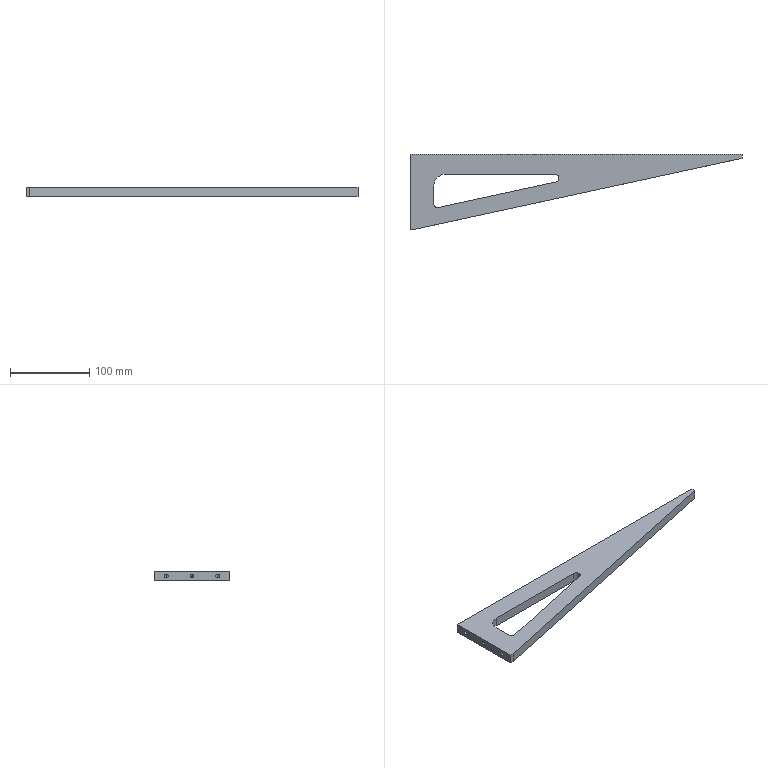Part | SolidWorks | features HoleWzd 2, Extrusion 1 | 1 solid | 41 faces | box 420 x 95 x 12 mm | volume 203565 mm3 | cylinder 17 | cone 14 | plane 10 | commonest cylinder face diameters 5 x14 10 x2 30 x1
STEP:
#1=CARTESIAN_POINT('',(45.,-15.,3.5));
#2=VERTEX_POINT('',#1);
#3=CARTESIAN_POINT('',(45.,-15.,8.5));
#4=VERTEX_POINT('',#3);
#5=CARTESIAN_POINT('',(45.,-15.,6.));
#6=DIRECTION('',(0.,1.,0.));
#7=DIRECTION('',(0.,0.,1.));
#8=AXIS2_PLACEMENT_3D('',#5,#6,#7);
#9=CIRCLE('',#8,2.5);
#10=EDGE_CURVE('',#2,#4,#9,.T.);
#11=ORIENTED_EDGE('',*,*,#10,.F.);
#12=CARTESIAN_POINT('',(45.,0.,3.5));
#13=VERTEX_POINT('',#12);
#14=CARTESIAN_POINT('',(45.,0.,3.5));
#15=DIRECTION('',(0.,1.,0.));
#16=VECTOR('',#15,1000.);
#17=LINE('',#14,#16);
#18=EDGE_CURVE('',#2,#13,#17,.T.);
#19=ORIENTED_EDGE('',*,*,#18,.T.);
#20=CARTESIAN_POINT('',(45.,0.,8.5));
#21=VERTEX_POINT('',#20);
#22=CARTESIAN_POINT('',(45.,0.,6.));
#23=DIRECTION('',(0.,1.,0.));
#24=DIRECTION('',(0.,0.,1.));
#25=AXIS2_PLACEMENT_3D('',#22,#23,#24);
#26=CIRCLE('',#25,2.5);
#27=EDGE_CURVE('',#13,#21,#26,.T.);
#28=ORIENTED_EDGE('',*,*,#27,.T.);
#29=CARTESIAN_POINT('',(45.,0.,8.5));
#30=DIRECTION('',(0.,1.,0.));
#31=VECTOR('',#30,1000.);
#32=LINE('',#29,#31);
#33=EDGE_CURVE('',#4,#21,#32,.T.);
#34=ORIENTED_EDGE('',*,*,#33,.F.);
#35=EDGE_LOOP('',(#11,#19,#28,#34));
#36=FACE_OUTER_BOUND('',#35,.T.);
#37=CARTESIAN_POINT('',(45.,0.,6.));
#38=DIRECTION('',(0.,1.,0.));
#39=DIRECTION('',(0.,0.,1.));
#40=AXIS2_PLACEMENT_3D('',#37,#38,#39);
#41=CYLINDRICAL_SURFACE('',#40,2.5);
#42=ADVANCED_FACE('',(#36),#41,.F.);
#43=CARTESIAN_POINT('',(45.,-16.502,6.));
#44=VERTEX_POINT('',#43);
#45=CARTESIAN_POINT('',(45.,-15.,8.5));
#46=DIRECTION('',(0.,0.515,0.8572));
#47=VECTOR('',#46,1000.);
#48=LINE('',#45,#47);
#49=EDGE_CURVE('',#44,#4,#48,.T.);
#50=ORIENTED_EDGE('',*,*,#49,.F.);
#51=CARTESIAN_POINT('',(45.,-15.,3.5));
#52=DIRECTION('',(0.,0.515,-0.8572));
#53=VECTOR('',#52,1000.);
#54=LINE('',#51,#53);
#55=EDGE_CURVE('',#44,#2,#54,.T.);
#56=ORIENTED_EDGE('',*,*,#55,.T.);
#57=ORIENTED_EDGE('',*,*,#10,.T.);
#58=EDGE_LOOP('',(#50,#56,#57));
#59=FACE_OUTER_BOUND('',#58,.T.);
#60=CARTESIAN_POINT('',(45.,-15.,6.));
#61=DIRECTION('',(0.,1.,0.));
#62=DIRECTION('',(0.,0.,1.));
#63=AXIS2_PLACEMENT_3D('',#60,#61,#62);
#64=CONICAL_SURFACE('',#63,2.5,1.03);
#65=ADVANCED_FACE('',(#59),#64,.F.);
#66=CARTESIAN_POINT('',(145.,-15.,3.5));
#67=VERTEX_POINT('',#66);
#68=CARTESIAN_POINT('',(145.,-15.,8.5));
#69=VERTEX_POINT('',#68);
#70=CARTESIAN_POINT('',(145.,-15.,6.));
#71=DIRECTION('',(0.,1.,0.));
#72=DIRECTION('',(0.,0.,1.));
#73=AXIS2_PLACEMENT_3D('',#70,#71,#72);
#74=CIRCLE('',#73,2.5);
#75=EDGE_CURVE('',#67,#69,#74,.T.);
#76=ORIENTED_EDGE('',*,*,#75,.F.);
#77=CARTESIAN_POINT('',(145.,0.,3.5));
#78=VERTEX_POINT('',#77);
#79=CARTESIAN_POINT('',(145.,0.,3.5));
#80=DIRECTION('',(0.,1.,0.));
#81=VECTOR('',#80,1000.);
#82=LINE('',#79,#81);
#83=EDGE_CURVE('',#67,#78,#82,.T.);
#84=ORIENTED_EDGE('',*,*,#83,.T.);
#85=CARTESIAN_POINT('',(145.,0.,8.5));
#86=VERTEX_POINT('',#85);
#87=CARTESIAN_POINT('',(145.,0.,6.));
#88=DIRECTION('',(0.,1.,0.));
#89=DIRECTION('',(0.,0.,1.));
#90=AXIS2_PLACEMENT_3D('',#87,#88,#89);
#91=CIRCLE('',#90,2.5);
#92=EDGE_CURVE('',#78,#86,#91,.T.);
#93=ORIENTED_EDGE('',*,*,#92,.T.);
#94=CARTESIAN_POINT('',(145.,0.,8.5));
#95=DIRECTION('',(0.,1.,0.));
#96=VECTOR('',#95,1000.);
#97=LINE('',#94,#96);
#98=EDGE_CURVE('',#69,#86,#97,.T.);
#99=ORIENTED_EDGE('',*,*,#98,.F.);
#100=EDGE_LOOP('',(#76,#84,#93,#99));
#101=FACE_OUTER_BOUND('',#100,.T.);
#102=CARTESIAN_POINT('',(145.,0.,6.));
#103=DIRECTION('',(0.,1.,0.));
#104=DIRECTION('',(0.,0.,1.));
#105=AXIS2_PLACEMENT_3D('',#102,#103,#104);
#106=CYLINDRICAL_SURFACE('',#105,2.5);
#107=ADVANCED_FACE('',(#101),#106,.F.);
#108=CARTESIAN_POINT('',(145.,-16.502,6.));
#109=VERTEX_POINT('',#108);
#110=CARTESIAN_POINT('',(145.,-15.,8.5));
#111=DIRECTION('',(0.,0.515,0.8572));
#112=VECTOR('',#111,1000.);
#113=LINE('',#110,#112);
#114=EDGE_CURVE('',#109,#69,#113,.T.);
#115=ORIENTED_EDGE('',*,*,#114,.F.);
#116=CARTESIAN_POINT('',(145.,-15.,3.5));
#117=DIRECTION('',(0.,0.515,-0.8572));
#118=VECTOR('',#117,1000.);
#119=LINE('',#116,#118);
#120=EDGE_CURVE('',#109,#67,#119,.T.);
#121=ORIENTED_EDGE('',*,*,#120,.T.);
#122=ORIENTED_EDGE('',*,*,#75,.T.);
#123=EDGE_LOOP('',(#115,#121,#122));
#124=FACE_OUTER_BOUND('',#123,.T.);
#125=CARTESIAN_POINT('',(145.,-15.,6.));
#126=DIRECTION('',(0.,1.,0.));
#127=DIRECTION('',(0.,0.,1.));
#128=AXIS2_PLACEMENT_3D('',#125,#126,#127);
#129=CONICAL_SURFACE('',#128,2.5,1.03);
#130=ADVANCED_FACE('',(#124),#129,.F.);
#131=CARTESIAN_POINT('',(245.,-15.,3.5));
#132=VERTEX_POINT('',#131);
#133=CARTESIAN_POINT('',(245.,-15.,8.5));
#134=VERTEX_POINT('',#133);
#135=CARTESIAN_POINT('',(245.,-15.,6.));
#136=DIRECTION('',(0.,1.,0.));
#137=DIRECTION('',(0.,0.,1.));
#138=AXIS2_PLACEMENT_3D('',#135,#136,#137);
#139=CIRCLE('',#138,2.5);
#140=EDGE_CURVE('',#132,#134,#139,.T.);
#141=ORIENTED_EDGE('',*,*,#140,.F.);
#142=CARTESIAN_POINT('',(245.,0.,3.5));
#143=VERTEX_POINT('',#142);
#144=CARTESIAN_POINT('',(245.,0.,3.5));
#145=DIRECTION('',(0.,1.,0.));
#146=VECTOR('',#145,1000.);
#147=LINE('',#144,#146);
#148=EDGE_CURVE('',#132,#143,#147,.T.);
#149=ORIENTED_EDGE('',*,*,#148,.T.);
#150=CARTESIAN_POINT('',(245.,0.,8.5));
#151=VERTEX_POINT('',#150);
#152=CARTESIAN_POINT('',(245.,0.,6.));
#153=DIRECTION('',(0.,1.,0.));
#154=DIRECTION('',(0.,0.,1.));
#155=AXIS2_PLACEMENT_3D('',#152,#153,#154);
#156=CIRCLE('',#155,2.5);
#157=EDGE_CURVE('',#143,#151,#156,.T.);
#158=ORIENTED_EDGE('',*,*,#157,.T.);
#159=CARTESIAN_POINT('',(245.,0.,8.5));
#160=DIRECTION('',(0.,1.,0.));
#161=VECTOR('',#160,1000.);
#162=LINE('',#159,#161);
#163=EDGE_CURVE('',#134,#151,#162,.T.);
#164=ORIENTED_EDGE('',*,*,#163,.F.);
#165=EDGE_LOOP('',(#141,#149,#158,#164));
#166=FACE_OUTER_BOUND('',#165,.T.);
#167=CARTESIAN_POINT('',(245.,0.,6.));
#168=DIRECTION('',(0.,1.,0.));
#169=DIRECTION('',(0.,0.,1.));
#170=AXIS2_PLACEMENT_3D('',#167,#168,#169);
#171=CYLINDRICAL_SURFACE('',#170,2.5);
#172=ADVANCED_FACE('',(#166),#171,.F.);
#173=CARTESIAN_POINT('',(245.,-16.502,6.));
#174=VERTEX_POINT('',#173);
#175=CARTESIAN_POINT('',(245.,-15.,8.5));
#176=DIRECTION('',(0.,0.515,0.8572));
#177=VECTOR('',#176,1000.);
#178=LINE('',#175,#177);
#179=EDGE_CURVE('',#174,#134,#178,.T.);
#180=ORIENTED_EDGE('',*,*,#179,.F.);
#181=CARTESIAN_POINT('',(245.,-15.,3.5));
#182=DIRECTION('',(0.,0.515,-0.8572));
#183=VECTOR('',#182,1000.);
#184=LINE('',#181,#183);
#185=EDGE_CURVE('',#174,#132,#184,.T.);
#186=ORIENTED_EDGE('',*,*,#185,.T.);
#187=ORIENTED_EDGE('',*,*,#140,.T.);
#188=EDGE_LOOP('',(#180,#186,#187));
#189=FACE_OUTER_BOUND('',#188,.T.);
#190=CARTESIAN_POINT('',(245.,-15.,6.));
#191=DIRECTION('',(0.,1.,0.));
#192=DIRECTION('',(0.,0.,1.));
#193=AXIS2_PLACEMENT_3D('',#190,#191,#192);
#194=CONICAL_SURFACE('',#193,2.5,1.03);
#195=ADVANCED_FACE('',(#189),#194,.F.);
#196=CARTESIAN_POINT('',(345.,-15.,3.5));
#197=VERTEX_POINT('',#196);
#198=CARTESIAN_POINT('',(345.,-15.,8.5));
#199=VERTEX_POINT('',#198);
#200=CARTESIAN_POINT('',(345.,-15.,6.));
#201=DIRECTION('',(0.,1.,0.));
#202=DIRECTION('',(0.,0.,1.));
#203=AXIS2_PLACEMENT_3D('',#200,#201,#202);
#204=CIRCLE('',#203,2.5);
#205=EDGE_CURVE('',#197,#199,#204,.T.);
#206=ORIENTED_EDGE('',*,*,#205,.F.);
#207=CARTESIAN_POINT('',(345.,0.,3.5));
#208=VERTEX_POINT('',#207);
#209=CARTESIAN_POINT('',(345.,0.,3.5));
#210=DIRECTION('',(0.,1.,0.));
#211=VECTOR('',#210,1000.);
#212=LINE('',#209,#211);
#213=EDGE_CURVE('',#197,#208,#212,.T.);
#214=ORIENTED_EDGE('',*,*,#213,.T.);
#215=CARTESIAN_POINT('',(345.,0.,8.5));
#216=VERTEX_POINT('',#215);
#217=CARTESIAN_POINT('',(345.,0.,6.));
#218=DIRECTION('',(0.,1.,0.));
#219=DIRECTION('',(0.,0.,1.));
#220=AXIS2_PLACEMENT_3D('',#217,#218,#219);
#221=CIRCLE('',#220,2.5);
#222=EDGE_CURVE('',#208,#216,#221,.T.);
#223=ORIENTED_EDGE('',*,*,#222,.T.);
#224=CARTESIAN_POINT('',(345.,0.,8.5));
#225=DIRECTION('',(0.,1.,0.));
#226=VECTOR('',#225,1000.);
#227=LINE('',#224,#226);
#228=EDGE_CURVE('',#199,#216,#227,.T.);
#229=ORIENTED_EDGE('',*,*,#228,.F.);
#230=EDGE_LOOP('',(#206,#214,#223,#229));
#231=FACE_OUTER_BOUND('',#230,.T.);
#232=CARTESIAN_POINT('',(345.,0.,6.));
#233=DIRECTION('',(0.,1.,0.));
#234=DIRECTION('',(0.,0.,1.));
#235=AXIS2_PLACEMENT_3D('',#232,#233,#234);
#236=CYLINDRICAL_SURFACE('',#235,2.5);
#237=ADVANCED_FACE('',(#231),#236,.F.);
#238=CARTESIAN_POINT('',(345.,-16.502,6.));
#239=VERTEX_POINT('',#238);
#240=CARTESIAN_POINT('',(345.,-15.,8.5));
#241=DIRECTION('',(0.,0.515,0.8572));
#242=VECTOR('',#241,1000.);
#243=LINE('',#240,#242);
#244=EDGE_CURVE('',#239,#199,#243,.T.);
#245=ORIENTED_EDGE('',*,*,#244,.F.);
#246=CARTESIAN_POINT('',(345.,-15.,3.5));
#247=DIRECTION('',(0.,0.515,-0.8572));
#248=VECTOR('',#247,1000.);
#249=LINE('',#246,#248);
#250=EDGE_CURVE('',#239,#197,#249,.T.);
#251=ORIENTED_EDGE('',*,*,#250,.T.);
#252=ORIENTED_EDGE('',*,*,#205,.T.);
#253=EDGE_LOOP('',(#245,#251,#252));
#254=FACE_OUTER_BOUND('',#253,.T.);
#255=CARTESIAN_POINT('',(345.,-15.,6.));
#256=DIRECTION('',(0.,1.,0.));
#257=DIRECTION('',(0.,0.,1.));
#258=AXIS2_PLACEMENT_3D('',#255,#256,#257);
#259=CONICAL_SURFACE('',#258,2.5,1.03);
#260=ADVANCED_FACE('',(#254),#259,.F.);
#261=CARTESIAN_POINT('',(15.,-15.,3.5));
#262=VERTEX_POINT('',#261);
#263=CARTESIAN_POINT('',(15.,-15.,8.5));
#264=VERTEX_POINT('',#263);
#265=CARTESIAN_POINT('',(15.,-15.,6.));
#266=DIRECTION('',(-1.,0.,0.));
#267=DIRECTION('',(0.,0.,1.));
#268=AXIS2_PLACEMENT_3D('',#265,#266,#267);
#269=CIRCLE('',#268,2.5);
#270=EDGE_CURVE('',#262,#264,#269,.T.);
#271=ORIENTED_EDGE('',*,*,#270,.F.);
#272=CARTESIAN_POINT('',(0.,-15.,3.5));
#273=VERTEX_POINT('',#272);
#274=CARTESIAN_POINT('',(0.,-15.,3.5));
#275=DIRECTION('',(-1.,0.,0.));
#276=VECTOR('',#275,1000.);
#277=LINE('',#274,#276);
#278=EDGE_CURVE('',#262,#273,#277,.T.);
#279=ORIENTED_EDGE('',*,*,#278,.T.);
#280=CARTESIAN_POINT('',(0.,-15.,8.5));
#281=VERTEX_POINT('',#280);
#282=CARTESIAN_POINT('',(0.,-15.,6.));
#283=DIRECTION('',(-1.,0.,0.));
#284=DIRECTION('',(0.,0.,1.));
#285=AXIS2_PLACEMENT_3D('',#282,#283,#284);
#286=CIRCLE('',#285,2.5);
#287=EDGE_CURVE('',#273,#281,#286,.T.);
#288=ORIENTED_EDGE('',*,*,#287,.T.);
#289=CARTESIAN_POINT('',(0.,-15.,8.5));
#290=DIRECTION('',(-1.,0.,0.));
#291=VECTOR('',#290,1000.);
#292=LINE('',#289,#291);
#293=EDGE_CURVE('',#264,#281,#292,.T.);
#294=ORIENTED_EDGE('',*,*,#293,.F.);
#295=EDGE_LOOP('',(#271,#279,#288,#294));
#296=FACE_OUTER_BOUND('',#295,.T.);
#297=CARTESIAN_POINT('',(0.,-15.,6.));
#298=DIRECTION('',(-1.,0.,0.));
#299=DIRECTION('',(0.,0.,1.));
#300=AXIS2_PLACEMENT_3D('',#297,#298,#299);
#301=CYLINDRICAL_SURFACE('',#300,2.5);
#302=ADVANCED_FACE('',(#296),#301,.F.);
#303=CARTESIAN_POINT('',(16.502,-15.,6.));
#304=VERTEX_POINT('',#303);
#305=CARTESIAN_POINT('',(15.,-15.,8.5));
#306=DIRECTION('',(-0.515,0.,0.8572));
#307=VECTOR('',#306,1000.);
#308=LINE('',#305,#307);
#309=EDGE_CURVE('',#304,#264,#308,.T.);
#310=ORIENTED_EDGE('',*,*,#309,.F.);
#311=CARTESIAN_POINT('',(15.,-15.,3.5));
#312=DIRECTION('',(-0.515,0.,-0.8572));
#313=VECTOR('',#312,1000.);
#314=LINE('',#311,#313);
#315=EDGE_CURVE('',#304,#262,#314,.T.);
#316=ORIENTED_EDGE('',*,*,#315,.T.);
#317=ORIENTED_EDGE('',*,*,#270,.T.);
#318=EDGE_LOOP('',(#310,#316,#317));
#319=FACE_OUTER_BOUND('',#318,.T.);
#320=CARTESIAN_POINT('',(15.,-15.,6.));
#321=DIRECTION('',(-1.,0.,0.));
#322=DIRECTION('',(0.,0.,1.));
#323=AXIS2_PLACEMENT_3D('',#320,#321,#322);
#324=CONICAL_SURFACE('',#323,2.5,1.03);
#325=ADVANCED_FACE('',(#319),#324,.F.);
#326=CARTESIAN_POINT('',(15.,-47.5,3.5));
#327=VERTEX_POINT('',#326);
#328=CARTESIAN_POINT('',(15.,-47.5,8.5));
#329=VERTEX_POINT('',#328);
#330=CARTESIAN_POINT('',(15.,-47.5,6.));
#331=DIRECTION('',(-1.,0.,0.));
#332=DIRECTION('',(0.,0.,1.));
#333=AXIS2_PLACEMENT_3D('',#330,#331,#332);
#334=CIRCLE('',#333,2.5);
#335=EDGE_CURVE('',#327,#329,#334,.T.);
#336=ORIENTED_EDGE('',*,*,#335,.F.);
#337=CARTESIAN_POINT('',(0.,-47.5,3.5));
#338=VERTEX_POINT('',#337);
#339=CARTESIAN_POINT('',(0.,-47.5,3.5));
#340=DIRECTION('',(-1.,0.,0.));
#341=VECTOR('',#340,1000.);
#342=LINE('',#339,#341);
#343=EDGE_CURVE('',#327,#338,#342,.T.);
#344=ORIENTED_EDGE('',*,*,#343,.T.);
#345=CARTESIAN_POINT('',(0.,-47.5,8.5));
#346=VERTEX_POINT('',#345);
#347=CARTESIAN_POINT('',(0.,-47.5,6.));
#348=DIRECTION('',(-1.,0.,0.));
#349=DIRECTION('',(0.,0.,1.));
#350=AXIS2_PLACEMENT_3D('',#347,#348,#349);
#351=CIRCLE('',#350,2.5);
#352=EDGE_CURVE('',#338,#346,#351,.T.);
#353=ORIENTED_EDGE('',*,*,#352,.T.);
#354=CARTESIAN_POINT('',(0.,-47.5,8.5));
#355=DIRECTION('',(-1.,0.,0.));
#356=VECTOR('',#355,1000.);
#357=LINE('',#354,#356);
#358=EDGE_CURVE('',#329,#346,#357,.T.);
#359=ORIENTED_EDGE('',*,*,#358,.F.);
#360=EDGE_LOOP('',(#336,#344,#353,#359));
#361=FACE_OUTER_BOUND('',#360,.T.);
#362=CARTESIAN_POINT('',(0.,-47.5,6.));
#363=DIRECTION('',(-1.,0.,0.));
#364=DIRECTION('',(0.,0.,1.));
#365=AXIS2_PLACEMENT_3D('',#362,#363,#364);
#366=CYLINDRICAL_SURFACE('',#365,2.5);
#367=ADVANCED_FACE('',(#361),#366,.F.);
#368=CARTESIAN_POINT('',(16.502,-47.5,6.));
#369=VERTEX_POINT('',#368);
#370=CARTESIAN_POINT('',(15.,-47.5,8.5));
#371=DIRECTION('',(-0.515,0.,0.8572));
#372=VECTOR('',#371,1000.);
#373=LINE('',#370,#372);
#374=EDGE_CURVE('',#369,#329,#373,.T.);
#375=ORIENTED_EDGE('',*,*,#374,.F.);
#376=CARTESIAN_POINT('',(15.,-47.5,3.5));
#377=DIRECTION('',(-0.515,0.,-0.8572));
#378=VECTOR('',#377,1000.);
#379=LINE('',#376,#378);
#380=EDGE_CURVE('',#369,#327,#379,.T.);
#381=ORIENTED_EDGE('',*,*,#380,.T.);
#382=ORIENTED_EDGE('',*,*,#335,.T.);
#383=EDGE_LOOP('',(#375,#381,#382));
#384=FACE_OUTER_BOUND('',#383,.T.);
#385=CARTESIAN_POINT('',(15.,-47.5,6.));
#386=DIRECTION('',(-1.,0.,0.));
#387=DIRECTION('',(0.,0.,1.));
#388=AXIS2_PLACEMENT_3D('',#385,#386,#387);
#389=CONICAL_SURFACE('',#388,2.5,1.03);
#390=ADVANCED_FACE('',(#384),#389,.F.);
#391=CARTESIAN_POINT('',(15.,-80.,3.5));
#392=VERTEX_POINT('',#391);
#393=CARTESIAN_POINT('',(15.,-80.,8.5));
#394=VERTEX_POINT('',#393);
#395=CARTESIAN_POINT('',(15.,-80.,6.));
#396=DIRECTION('',(-1.,0.,0.));
#397=DIRECTION('',(0.,0.,1.));
#398=AXIS2_PLACEMENT_3D('',#395,#396,#397);
#399=CIRCLE('',#398,2.5);
#400=EDGE_CURVE('',#392,#394,#399,.T.);
#401=ORIENTED_EDGE('',*,*,#400,.F.);
#402=CARTESIAN_POINT('',(0.,-80.,3.5));
#403=VERTEX_POINT('',#402);
#404=CARTESIAN_POINT('',(0.,-80.,3.5));
#405=DIRECTION('',(-1.,0.,0.));
#406=VECTOR('',#405,1000.);
#407=LINE('',#404,#406);
#408=EDGE_CURVE('',#392,#403,#407,.T.);
#409=ORIENTED_EDGE('',*,*,#408,.T.);
#410=CARTESIAN_POINT('',(0.,-80.,8.5));
#411=VERTEX_POINT('',#410);
#412=CARTESIAN_POINT('',(0.,-80.,6.));
#413=DIRECTION('',(-1.,0.,0.));
#414=DIRECTION('',(0.,0.,1.));
#415=AXIS2_PLACEMENT_3D('',#412,#413,#414);
#416=CIRCLE('',#415,2.5);
#417=EDGE_CURVE('',#403,#411,#416,.T.);
#418=ORIENTED_EDGE('',*,*,#417,.T.);
#419=CARTESIAN_POINT('',(0.,-80.,8.5));
#420=DIRECTION('',(-1.,0.,0.));
#421=VECTOR('',#420,1000.);
#422=LINE('',#419,#421);
#423=EDGE_CURVE('',#394,#411,#422,.T.);
#424=ORIENTED_EDGE('',*,*,#423,.F.);
#425=EDGE_LOOP('',(#401,#409,#418,#424));
#426=FACE_OUTER_BOUND('',#425,.T.);
#427=CARTESIAN_POINT('',(0.,-80.,6.));
#428=DIRECTION('',(-1.,0.,0.));
#429=DIRECTION('',(0.,0.,1.));
#430=AXIS2_PLACEMENT_3D('',#427,#428,#429);
#431=CYLINDRICAL_SURFACE('',#430,2.5);
#432=ADVANCED_FACE('',(#426),#431,.F.);
#433=CARTESIAN_POINT('',(16.502,-80.,6.));
#434=VERTEX_POINT('',#433);
#435=CARTESIAN_POINT('',(15.,-80.,8.5));
#436=DIRECTION('',(-0.515,0.,0.8572));
#437=VECTOR('',#436,1000.);
#438=LINE('',#435,#437);
#439=EDGE_CURVE('',#434,#394,#438,.T.);
#440=ORIENTED_EDGE('',*,*,#439,.F.);
#441=CARTESIAN_POINT('',(15.,-80.,3.5));
#442=DIRECTION('',(-0.515,0.,-0.8572));
#443=VECTOR('',#442,1000.);
#444=LINE('',#441,#443);
#445=EDGE_CURVE('',#434,#392,#444,.T.);
#446=ORIENTED_EDGE('',*,*,#445,.T.);
#447=ORIENTED_EDGE('',*,*,#400,.T.);
#448=EDGE_LOOP('',(#440,#446,#447));
#449=FACE_OUTER_BOUND('',#448,.T.);
#450=CARTESIAN_POINT('',(15.,-80.,6.));
#451=DIRECTION('',(-1.,0.,0.));
#452=DIRECTION('',(0.,0.,1.));
#453=AXIS2_PLACEMENT_3D('',#450,#451,#452);
#454=CONICAL_SURFACE('',#453,2.5,1.03);
#455=ADVANCED_FACE('',(#449),#454,.F.);
#456=CARTESIAN_POINT('',(420.,0.,12.));
#457=VERTEX_POINT('',#456);
#458=CARTESIAN_POINT('',(0.,0.,12.));
#459=VERTEX_POINT('',#458);
#460=CARTESIAN_POINT('',(0.,0.,12.));
#461=DIRECTION('',(-1.,0.,0.));
#462=VECTOR('',#461,1000.);
#463=LINE('',#460,#462);
#464=EDGE_CURVE('',#457,#459,#463,.T.);
#465=ORIENTED_EDGE('',*,*,#464,.T.);
#466=CARTESIAN_POINT('',(0.,-95.,12.));
#467=VERTEX_POINT('',#466);
#468=CARTESIAN_POINT('',(0.,-95.,12.));
#469=DIRECTION('',(0.,-1.,0.));
#470=VECTOR('',#469,1000.);
#471=LINE('',#468,#470);
#472=EDGE_CURVE('',#459,#467,#471,.T.);
#473=ORIENTED_EDGE('',*,*,#472,.T.);
#474=CARTESIAN_POINT('',(5.,-95.,12.));
#475=VERTEX_POINT('',#474);
#476=CARTESIAN_POINT('',(5.,-95.,12.));
#477=DIRECTION('',(1.,0.,0.));
#478=VECTOR('',#477,1000.);
#479=LINE('',#476,#478);
#480=EDGE_CURVE('',#467,#475,#479,.T.);
#481=ORIENTED_EDGE('',*,*,#480,.T.);
#482=CARTESIAN_POINT('',(420.,-5.,12.));
#483=VERTEX_POINT('',#482);
#484=CARTESIAN_POINT('',(420.,-5.,12.));
#485=DIRECTION('',(0.9773,0.2119,0.));
#486=VECTOR('',#485,1000.);
#487=LINE('',#484,#486);
#488=EDGE_CURVE('',#475,#483,#487,.T.);
#489=ORIENTED_EDGE('',*,*,#488,.T.);
#490=CARTESIAN_POINT('',(420.,0.,12.));
#491=DIRECTION('',(0.,1.,0.));
#492=VECTOR('',#491,1000.);
#493=LINE('',#490,#492);
#494=EDGE_CURVE('',#483,#457,#493,.T.);
#495=ORIENTED_EDGE('',*,*,#494,.T.);
#496=EDGE_LOOP('',(#465,#473,#481,#489,#495));
#497=FACE_OUTER_BOUND('',#496,.T.);
#498=CARTESIAN_POINT('',(45.,-25.,12.));
#499=VERTEX_POINT('',#498);
#500=CARTESIAN_POINT('',(30.,-40.,12.));
#501=VERTEX_POINT('',#500);
#502=CARTESIAN_POINT('',(45.,-40.,12.));
#503=DIRECTION('',(0.,0.,1.));
#504=DIRECTION('',(1.,0.,0.));
#505=AXIS2_PLACEMENT_3D('',#502,#503,#504);
#506=CIRCLE('',#505,15.);
#507=EDGE_CURVE('',#499,#501,#506,.T.);
#508=ORIENTED_EDGE('',*,*,#507,.F.);
#509=CARTESIAN_POINT('',(183.353,-25.,12.));
#510=VERTEX_POINT('',#509);
#511=CARTESIAN_POINT('',(45.,-25.,12.));
#512=DIRECTION('',(-1.,0.,0.));
#513=VECTOR('',#512,1000.);
#514=LINE('',#511,#513);
#515=EDGE_CURVE('',#510,#499,#514,.T.);
#516=ORIENTED_EDGE('',*,*,#515,.F.);
#517=CARTESIAN_POINT('',(184.413,-34.886,12.));
#518=VERTEX_POINT('',#517);
#519=CARTESIAN_POINT('',(183.353,-30.,12.));
#520=DIRECTION('',(0.,0.,1.));
#521=DIRECTION('',(-1.,0.,0.));
#522=AXIS2_PLACEMENT_3D('',#519,#520,#521);
#523=CIRCLE('',#522,5.);
#524=EDGE_CURVE('',#518,#510,#523,.T.);
#525=ORIENTED_EDGE('',*,*,#524,.F.);
#526=CARTESIAN_POINT('',(36.06,-67.059,12.));
#527=VERTEX_POINT('',#526);
#528=CARTESIAN_POINT('',(184.413,-34.886,12.));
#529=DIRECTION('',(0.9773,0.2119,0.));
#530=VECTOR('',#529,1000.);
#531=LINE('',#528,#530);
#532=EDGE_CURVE('',#527,#518,#531,.T.);
#533=ORIENTED_EDGE('',*,*,#532,.F.);
#534=CARTESIAN_POINT('',(30.,-62.173,12.));
#535=VERTEX_POINT('',#534);
#536=CARTESIAN_POINT('',(35.,-62.173,12.));
#537=DIRECTION('',(0.,0.,1.));
#538=DIRECTION('',(1.,0.,0.));
#539=AXIS2_PLACEMENT_3D('',#536,#537,#538);
#540=CIRCLE('',#539,5.);
#541=EDGE_CURVE('',#535,#527,#540,.T.);
#542=ORIENTED_EDGE('',*,*,#541,.F.);
#543=CARTESIAN_POINT('',(30.,-62.173,12.));
#544=DIRECTION('',(0.,-1.,0.));
#545=VECTOR('',#544,1000.);
#546=LINE('',#543,#545);
#547=EDGE_CURVE('',#501,#535,#546,.T.);
#548=ORIENTED_EDGE('',*,*,#547,.F.);
#549=EDGE_LOOP('',(#508,#516,#525,#533,#542,#548));
#550=FACE_BOUND('',#549,.T.);
#551=CARTESIAN_POINT('',(0.,0.,12.));
#552=DIRECTION('',(0.,0.,-1.));
#553=DIRECTION('',(-1.,0.,0.));
#554=AXIS2_PLACEMENT_3D('',#551,#552,#553);
#555=PLANE('',#554);
#556=ADVANCED_FACE('',(#497,#550),#555,.F.);
#557=CARTESIAN_POINT('',(420.,0.,0.));
#558=VERTEX_POINT('',#557);
#559=CARTESIAN_POINT('',(0.,0.,0.));
#560=VERTEX_POINT('',#559);
#561=CARTESIAN_POINT('',(0.,0.,0.));
#562=DIRECTION('',(-1.,0.,0.));
#563=VECTOR('',#562,1000.);
#564=LINE('',#561,#563);
#565=EDGE_CURVE('',#558,#560,#564,.T.);
#566=ORIENTED_EDGE('',*,*,#565,.F.);
#567=CARTESIAN_POINT('',(420.,-5.,0.));
#568=VERTEX_POINT('',#567);
#569=CARTESIAN_POINT('',(420.,0.,0.));
#570=DIRECTION('',(0.,1.,0.));
#571=VECTOR('',#570,1000.);
#572=LINE('',#569,#571);
#573=EDGE_CURVE('',#568,#558,#572,.T.);
#574=ORIENTED_EDGE('',*,*,#573,.F.);
#575=CARTESIAN_POINT('',(5.,-95.,0.));
#576=VERTEX_POINT('',#575);
#577=CARTESIAN_POINT('',(420.,-5.,0.));
#578=DIRECTION('',(0.9773,0.2119,0.));
#579=VECTOR('',#578,1000.);
#580=LINE('',#577,#579);
#581=EDGE_CURVE('',#576,#568,#580,.T.);
#582=ORIENTED_EDGE('',*,*,#581,.F.);
#583=CARTESIAN_POINT('',(0.,-95.,0.));
#584=VERTEX_POINT('',#583);
#585=CARTESIAN_POINT('',(5.,-95.,0.));
#586=DIRECTION('',(1.,0.,0.));
#587=VECTOR('',#586,1000.);
#588=LINE('',#585,#587);
#589=EDGE_CURVE('',#584,#576,#588,.T.);
#590=ORIENTED_EDGE('',*,*,#589,.F.);
#591=CARTESIAN_POINT('',(0.,-95.,0.));
#592=DIRECTION('',(0.,-1.,0.));
#593=VECTOR('',#592,1000.);
#594=LINE('',#591,#593);
#595=EDGE_CURVE('',#560,#584,#594,.T.);
#596=ORIENTED_EDGE('',*,*,#595,.F.);
#597=EDGE_LOOP('',(#566,#574,#582,#590,#596));
#598=FACE_OUTER_BOUND('',#597,.T.);
#599=CARTESIAN_POINT('',(183.353,-25.,0.));
#600=VERTEX_POINT('',#599);
#601=CARTESIAN_POINT('',(45.,-25.,0.));
#602=VERTEX_POINT('',#601);
#603=CARTESIAN_POINT('',(45.,-25.,0.));
#604=DIRECTION('',(-1.,0.,0.));
#605=VECTOR('',#604,1000.);
#606=LINE('',#603,#605);
#607=EDGE_CURVE('',#600,#602,#606,.T.);
#608=ORIENTED_EDGE('',*,*,#607,.T.);
#609=CARTESIAN_POINT('',(30.,-40.,0.));
#610=VERTEX_POINT('',#609);
#611=CARTESIAN_POINT('',(45.,-40.,0.));
#612=DIRECTION('',(0.,0.,1.));
#613=DIRECTION('',(1.,0.,0.));
#614=AXIS2_PLACEMENT_3D('',#611,#612,#613);
#615=CIRCLE('',#614,15.);
#616=EDGE_CURVE('',#602,#610,#615,.T.);
#617=ORIENTED_EDGE('',*,*,#616,.T.);
#618=CARTESIAN_POINT('',(30.,-62.173,0.));
#619=VERTEX_POINT('',#618);
#620=CARTESIAN_POINT('',(30.,-62.173,0.));
#621=DIRECTION('',(0.,-1.,0.));
#622=VECTOR('',#621,1000.);
#623=LINE('',#620,#622);
#624=EDGE_CURVE('',#610,#619,#623,.T.);
#625=ORIENTED_EDGE('',*,*,#624,.T.);
#626=CARTESIAN_POINT('',(36.06,-67.059,0.));
#627=VERTEX_POINT('',#626);
#628=CARTESIAN_POINT('',(35.,-62.173,0.));
#629=DIRECTION('',(0.,0.,1.));
#630=DIRECTION('',(1.,0.,0.));
#631=AXIS2_PLACEMENT_3D('',#628,#629,#630);
#632=CIRCLE('',#631,5.);
#633=EDGE_CURVE('',#619,#627,#632,.T.);
#634=ORIENTED_EDGE('',*,*,#633,.T.);
#635=CARTESIAN_POINT('',(184.413,-34.886,0.));
#636=VERTEX_POINT('',#635);
#637=CARTESIAN_POINT('',(184.413,-34.886,0.));
#638=DIRECTION('',(0.9773,0.2119,0.));
#639=VECTOR('',#638,1000.);
#640=LINE('',#637,#639);
#641=EDGE_CURVE('',#627,#636,#640,.T.);
#642=ORIENTED_EDGE('',*,*,#641,.T.);
#643=CARTESIAN_POINT('',(183.353,-30.,0.));
#644=DIRECTION('',(0.,0.,1.));
#645=DIRECTION('',(-1.,0.,0.));
#646=AXIS2_PLACEMENT_3D('',#643,#644,#645);
#647=CIRCLE('',#646,5.);
#648=EDGE_CURVE('',#636,#600,#647,.T.);
#649=ORIENTED_EDGE('',*,*,#648,.T.);
#650=EDGE_LOOP('',(#608,#617,#625,#634,#642,#649));
#651=FACE_BOUND('',#650,.T.);
#652=CARTESIAN_POINT('',(0.,0.,0.));
#653=DIRECTION('',(0.,0.,-1.));
#654=DIRECTION('',(-1.,0.,0.));
#655=AXIS2_PLACEMENT_3D('',#652,#653,#654);
#656=PLANE('',#655);
#657=ADVANCED_FACE('',(#598,#651),#656,.T.);
#658=CARTESIAN_POINT('',(45.,0.,6.));
#659=DIRECTION('',(0.,1.,0.));
#660=DIRECTION('',(0.,0.,1.));
#661=AXIS2_PLACEMENT_3D('',#658,#659,#660);
#662=CIRCLE('',#661,2.5);
#663=EDGE_CURVE('',#21,#13,#662,.T.);
#664=ORIENTED_EDGE('',*,*,#663,.F.);
#665=ORIENTED_EDGE('',*,*,#27,.F.);
#666=EDGE_LOOP('',(#664,#665));
#667=FACE_BOUND('',#666,.T.);
#668=CARTESIAN_POINT('',(145.,0.,6.));
#669=DIRECTION('',(0.,1.,0.));
#670=DIRECTION('',(0.,0.,1.));
#671=AXIS2_PLACEMENT_3D('',#668,#669,#670);
#672=CIRCLE('',#671,2.5);
#673=EDGE_CURVE('',#86,#78,#672,.T.);
#674=ORIENTED_EDGE('',*,*,#673,.F.);
#675=ORIENTED_EDGE('',*,*,#92,.F.);
#676=EDGE_LOOP('',(#674,#675));
#677=FACE_BOUND('',#676,.T.);
#678=CARTESIAN_POINT('',(245.,0.,6.));
#679=DIRECTION('',(0.,1.,0.));
#680=DIRECTION('',(0.,0.,1.));
#681=AXIS2_PLACEMENT_3D('',#678,#679,#680);
#682=CIRCLE('',#681,2.5);
#683=EDGE_CURVE('',#151,#143,#682,.T.);
#684=ORIENTED_EDGE('',*,*,#683,.F.);
#685=ORIENTED_EDGE('',*,*,#157,.F.);
#686=EDGE_LOOP('',(#684,#685));
#687=FACE_BOUND('',#686,.T.);
#688=CARTESIAN_POINT('',(345.,0.,6.));
#689=DIRECTION('',(0.,1.,0.));
#690=DIRECTION('',(0.,0.,1.));
#691=AXIS2_PLACEMENT_3D('',#688,#689,#690);
#692=CIRCLE('',#691,2.5);
#693=EDGE_CURVE('',#216,#208,#692,.T.);
#694=ORIENTED_EDGE('',*,*,#693,.F.);
#695=ORIENTED_EDGE('',*,*,#222,.F.);
#696=EDGE_LOOP('',(#694,#695));
#697=FACE_BOUND('',#696,.T.);
#698=ORIENTED_EDGE('',*,*,#565,.T.);
#699=CARTESIAN_POINT('',(0.,0.,12.));
#700=DIRECTION('',(0.,0.,-1.));
#701=VECTOR('',#700,1000.);
#702=LINE('',#699,#701);
#703=EDGE_CURVE('',#459,#560,#702,.T.);
#704=ORIENTED_EDGE('',*,*,#703,.F.);
#705=ORIENTED_EDGE('',*,*,#464,.F.);
#706=CARTESIAN_POINT('',(420.,0.,12.));
#707=DIRECTION('',(0.,0.,-1.));
#708=VECTOR('',#707,1000.);
#709=LINE('',#706,#708);
#710=EDGE_CURVE('',#457,#558,#709,.T.);
#711=ORIENTED_EDGE('',*,*,#710,.T.);
#712=EDGE_LOOP('',(#698,#704,#705,#711));
#713=FACE_OUTER_BOUND('',#712,.T.);
#714=CARTESIAN_POINT('',(0.,0.,12.));
#715=DIRECTION('',(0.,-1.,0.));
#716=DIRECTION('',(0.,0.,-1.));
#717=AXIS2_PLACEMENT_3D('',#714,#715,#716);
#718=PLANE('',#717);
#719=ADVANCED_FACE('',(#667,#677,#687,#697,#713),#718,.F.);
#720=CARTESIAN_POINT('',(0.,-15.,6.));
#721=DIRECTION('',(-1.,0.,0.));
#722=DIRECTION('',(0.,0.,1.));
#723=AXIS2_PLACEMENT_3D('',#720,#721,#722);
#724=CIRCLE('',#723,2.5);
#725=EDGE_CURVE('',#281,#273,#724,.T.);
#726=ORIENTED_EDGE('',*,*,#725,.F.);
#727=ORIENTED_EDGE('',*,*,#287,.F.);
#728=EDGE_LOOP('',(#726,#727));
#729=FACE_BOUND('',#728,.T.);
#730=CARTESIAN_POINT('',(0.,-47.5,6.));
#731=DIRECTION('',(-1.,0.,0.));
#732=DIRECTION('',(0.,0.,1.));
#733=AXIS2_PLACEMENT_3D('',#730,#731,#732);
#734=CIRCLE('',#733,2.5);
#735=EDGE_CURVE('',#346,#338,#734,.T.);
#736=ORIENTED_EDGE('',*,*,#735,.F.);
#737=ORIENTED_EDGE('',*,*,#352,.F.);
#738=EDGE_LOOP('',(#736,#737));
#739=FACE_BOUND('',#738,.T.);
#740=CARTESIAN_POINT('',(0.,-80.,6.));
#741=DIRECTION('',(-1.,0.,0.));
#742=DIRECTION('',(0.,0.,1.));
#743=AXIS2_PLACEMENT_3D('',#740,#741,#742);
#744=CIRCLE('',#743,2.5);
#745=EDGE_CURVE('',#411,#403,#744,.T.);
#746=ORIENTED_EDGE('',*,*,#745,.F.);
#747=ORIENTED_EDGE('',*,*,#417,.F.);
#748=EDGE_LOOP('',(#746,#747));
#749=FACE_BOUND('',#748,.T.);
#750=ORIENTED_EDGE('',*,*,#595,.T.);
#751=CARTESIAN_POINT('',(0.,-95.,12.));
#752=DIRECTION('',(0.,0.,-1.));
#753=VECTOR('',#752,1000.);
#754=LINE('',#751,#753);
#755=EDGE_CURVE('',#467,#584,#754,.T.);
#756=ORIENTED_EDGE('',*,*,#755,.F.);
#757=ORIENTED_EDGE('',*,*,#472,.F.);
#758=ORIENTED_EDGE('',*,*,#703,.T.);
#759=EDGE_LOOP('',(#750,#756,#757,#758));
#760=FACE_OUTER_BOUND('',#759,.T.);
#761=CARTESIAN_POINT('',(0.,-95.,12.));
#762=DIRECTION('',(1.,0.,0.));
#763=DIRECTION('',(0.,0.,-1.));
#764=AXIS2_PLACEMENT_3D('',#761,#762,#763);
#765=PLANE('',#764);
#766=ADVANCED_FACE('',(#729,#739,#749,#760),#765,.F.);
#767=ORIENTED_EDGE('',*,*,#589,.T.);
#768=CARTESIAN_POINT('',(5.,-95.,12.));
#769=DIRECTION('',(0.,0.,-1.));
#770=VECTOR('',#769,1000.);
#771=LINE('',#768,#770);
#772=EDGE_CURVE('',#475,#576,#771,.T.);
#773=ORIENTED_EDGE('',*,*,#772,.F.);
#774=ORIENTED_EDGE('',*,*,#480,.F.);
#775=ORIENTED_EDGE('',*,*,#755,.T.);
#776=EDGE_LOOP('',(#767,#773,#774,#775));
#777=FACE_OUTER_BOUND('',#776,.T.);
#778=CARTESIAN_POINT('',(5.,-95.,12.));
#779=DIRECTION('',(0.,1.,0.));
#780=DIRECTION('',(-1.,0.,0.));
#781=AXIS2_PLACEMENT_3D('',#778,#779,#780);
#782=PLANE('',#781);
#783=ADVANCED_FACE('',(#777),#782,.F.);
#784=ORIENTED_EDGE('',*,*,#581,.T.);
#785=CARTESIAN_POINT('',(420.,-5.,12.));
#786=DIRECTION('',(0.,0.,-1.));
#787=VECTOR('',#786,1000.);
#788=LINE('',#785,#787);
#789=EDGE_CURVE('',#483,#568,#788,.T.);
#790=ORIENTED_EDGE('',*,*,#789,.F.);
#791=ORIENTED_EDGE('',*,*,#488,.F.);
#792=ORIENTED_EDGE('',*,*,#772,.T.);
#793=EDGE_LOOP('',(#784,#790,#791,#792));
#794=FACE_OUTER_BOUND('',#793,.T.);
#795=CARTESIAN_POINT('',(420.,-5.,12.));
#796=DIRECTION('',(-0.2119,0.9773,0.));
#797=DIRECTION('',(-0.9773,-0.2119,0.));
#798=AXIS2_PLACEMENT_3D('',#795,#796,#797);
#799=PLANE('',#798);
#800=ADVANCED_FACE('',(#794),#799,.F.);
#801=ORIENTED_EDGE('',*,*,#573,.T.);
#802=ORIENTED_EDGE('',*,*,#710,.F.);
#803=ORIENTED_EDGE('',*,*,#494,.F.);
#804=ORIENTED_EDGE('',*,*,#789,.T.);
#805=EDGE_LOOP('',(#801,#802,#803,#804));
#806=FACE_OUTER_BOUND('',#805,.T.);
#807=CARTESIAN_POINT('',(420.,0.,12.));
#808=DIRECTION('',(-1.,0.,0.));
#809=DIRECTION('',(0.,0.,1.));
#810=AXIS2_PLACEMENT_3D('',#807,#808,#809);
#811=PLANE('',#810);
#812=ADVANCED_FACE('',(#806),#811,.F.);
#813=ORIENTED_EDGE('',*,*,#616,.F.);
#814=CARTESIAN_POINT('',(45.,-25.,12.));
#815=DIRECTION('',(0.,0.,-1.));
#816=VECTOR('',#815,1000.);
#817=LINE('',#814,#816);
#818=EDGE_CURVE('',#499,#602,#817,.T.);
#819=ORIENTED_EDGE('',*,*,#818,.F.);
#820=ORIENTED_EDGE('',*,*,#507,.T.);
#821=CARTESIAN_POINT('',(30.,-40.,12.));
#822=DIRECTION('',(0.,0.,-1.));
#823=VECTOR('',#822,1000.);
#824=LINE('',#821,#823);
#825=EDGE_CURVE('',#501,#610,#824,.T.);
#826=ORIENTED_EDGE('',*,*,#825,.T.);
#827=EDGE_LOOP('',(#813,#819,#820,#826));
#828=FACE_OUTER_BOUND('',#827,.T.);
#829=CARTESIAN_POINT('',(45.,-40.,12.));
#830=DIRECTION('',(0.,0.,-1.));
#831=DIRECTION('',(-1.,0.,0.));
#832=AXIS2_PLACEMENT_3D('',#829,#830,#831);
#833=CYLINDRICAL_SURFACE('',#832,15.);
#834=ADVANCED_FACE('',(#828),#833,.F.);
#835=ORIENTED_EDGE('',*,*,#624,.F.);
#836=ORIENTED_EDGE('',*,*,#825,.F.);
#837=ORIENTED_EDGE('',*,*,#547,.T.);
#838=CARTESIAN_POINT('',(30.,-62.173,12.));
#839=DIRECTION('',(0.,0.,-1.));
#840=VECTOR('',#839,1000.);
#841=LINE('',#838,#840);
#842=EDGE_CURVE('',#535,#619,#841,.T.);
#843=ORIENTED_EDGE('',*,*,#842,.T.);
#844=EDGE_LOOP('',(#835,#836,#837,#843));
#845=FACE_OUTER_BOUND('',#844,.T.);
#846=CARTESIAN_POINT('',(30.,-62.173,12.));
#847=DIRECTION('',(1.,0.,0.));
#848=DIRECTION('',(0.,1.,0.));
#849=AXIS2_PLACEMENT_3D('',#846,#847,#848);
#850=PLANE('',#849);
#851=ADVANCED_FACE('',(#845),#850,.T.);
#852=ORIENTED_EDGE('',*,*,#633,.F.);
#853=ORIENTED_EDGE('',*,*,#842,.F.);
#854=ORIENTED_EDGE('',*,*,#541,.T.);
#855=CARTESIAN_POINT('',(36.06,-67.059,12.));
#856=DIRECTION('',(0.,0.,-1.));
#857=VECTOR('',#856,1000.);
#858=LINE('',#855,#857);
#859=EDGE_CURVE('',#527,#627,#858,.T.);
#860=ORIENTED_EDGE('',*,*,#859,.T.);
#861=EDGE_LOOP('',(#852,#853,#854,#860));
#862=FACE_OUTER_BOUND('',#861,.T.);
#863=CARTESIAN_POINT('',(35.,-62.173,12.));
#864=DIRECTION('',(0.,0.,-1.));
#865=DIRECTION('',(-1.,0.,0.));
#866=AXIS2_PLACEMENT_3D('',#863,#864,#865);
#867=CYLINDRICAL_SURFACE('',#866,5.);
#868=ADVANCED_FACE('',(#862),#867,.F.);
#869=ORIENTED_EDGE('',*,*,#641,.F.);
#870=ORIENTED_EDGE('',*,*,#859,.F.);
#871=ORIENTED_EDGE('',*,*,#532,.T.);
#872=CARTESIAN_POINT('',(184.413,-34.886,12.));
#873=DIRECTION('',(0.,0.,-1.));
#874=VECTOR('',#873,1000.);
#875=LINE('',#872,#874);
#876=EDGE_CURVE('',#518,#636,#875,.T.);
#877=ORIENTED_EDGE('',*,*,#876,.T.);
#878=EDGE_LOOP('',(#869,#870,#871,#877));
#879=FACE_OUTER_BOUND('',#878,.T.);
#880=CARTESIAN_POINT('',(184.413,-34.886,12.));
#881=DIRECTION('',(-0.2119,0.9773,0.));
#882=DIRECTION('',(-0.9773,-0.2119,0.));
#883=AXIS2_PLACEMENT_3D('',#880,#881,#882);
#884=PLANE('',#883);
#885=ADVANCED_FACE('',(#879),#884,.T.);
#886=ORIENTED_EDGE('',*,*,#648,.F.);
#887=ORIENTED_EDGE('',*,*,#876,.F.);
#888=ORIENTED_EDGE('',*,*,#524,.T.);
#889=CARTESIAN_POINT('',(183.353,-25.,12.));
#890=DIRECTION('',(0.,0.,-1.));
#891=VECTOR('',#890,1000.);
#892=LINE('',#889,#891);
#893=EDGE_CURVE('',#510,#600,#892,.T.);
#894=ORIENTED_EDGE('',*,*,#893,.T.);
#895=EDGE_LOOP('',(#886,#887,#888,#894));
#896=FACE_OUTER_BOUND('',#895,.T.);
#897=CARTESIAN_POINT('',(183.353,-30.,12.));
#898=DIRECTION('',(0.,0.,-1.));
#899=DIRECTION('',(-1.,0.,0.));
#900=AXIS2_PLACEMENT_3D('',#897,#898,#899);
#901=CYLINDRICAL_SURFACE('',#900,5.);
#902=ADVANCED_FACE('',(#896),#901,.F.);
#903=ORIENTED_EDGE('',*,*,#607,.F.);
#904=ORIENTED_EDGE('',*,*,#893,.F.);
#905=ORIENTED_EDGE('',*,*,#515,.T.);
#906=ORIENTED_EDGE('',*,*,#818,.T.);
#907=EDGE_LOOP('',(#903,#904,#905,#906));
#908=FACE_OUTER_BOUND('',#907,.T.);
#909=CARTESIAN_POINT('',(45.,-25.,12.));
#910=DIRECTION('',(0.,-1.,0.));
#911=DIRECTION('',(1.,0.,0.));
#912=AXIS2_PLACEMENT_3D('',#909,#910,#911);
#913=PLANE('',#912);
#914=ADVANCED_FACE('',(#908),#913,.T.);
#915=ORIENTED_EDGE('',*,*,#445,.F.);
#916=ORIENTED_EDGE('',*,*,#439,.T.);
#917=CARTESIAN_POINT('',(15.,-80.,6.));
#918=DIRECTION('',(-1.,0.,0.));
#919=DIRECTION('',(0.,0.,1.));
#920=AXIS2_PLACEMENT_3D('',#917,#918,#919);
#921=CIRCLE('',#920,2.5);
#922=EDGE_CURVE('',#394,#392,#921,.T.);
#923=ORIENTED_EDGE('',*,*,#922,.T.);
#924=EDGE_LOOP('',(#915,#916,#923));
#925=FACE_OUTER_BOUND('',#924,.T.);
#926=CARTESIAN_POINT('',(15.,-80.,6.));
#927=DIRECTION('',(-1.,0.,0.));
#928=DIRECTION('',(0.,0.,1.));
#929=AXIS2_PLACEMENT_3D('',#926,#927,#928);
#930=CONICAL_SURFACE('',#929,2.5,1.03);
#931=ADVANCED_FACE('',(#925),#930,.F.);
#932=ORIENTED_EDGE('',*,*,#408,.F.);
#933=ORIENTED_EDGE('',*,*,#922,.F.);
#934=ORIENTED_EDGE('',*,*,#423,.T.);
#935=ORIENTED_EDGE('',*,*,#745,.T.);
#936=EDGE_LOOP('',(#932,#933,#934,#935));
#937=FACE_OUTER_BOUND('',#936,.T.);
#938=CARTESIAN_POINT('',(0.,-80.,6.));
#939=DIRECTION('',(-1.,0.,0.));
#940=DIRECTION('',(0.,0.,1.));
#941=AXIS2_PLACEMENT_3D('',#938,#939,#940);
#942=CYLINDRICAL_SURFACE('',#941,2.5);
#943=ADVANCED_FACE('',(#937),#942,.F.);
#944=ORIENTED_EDGE('',*,*,#380,.F.);
#945=ORIENTED_EDGE('',*,*,#374,.T.);
#946=CARTESIAN_POINT('',(15.,-47.5,6.));
#947=DIRECTION('',(-1.,0.,0.));
#948=DIRECTION('',(0.,0.,1.));
#949=AXIS2_PLACEMENT_3D('',#946,#947,#948);
#950=CIRCLE('',#949,2.5);
#951=EDGE_CURVE('',#329,#327,#950,.T.);
#952=ORIENTED_EDGE('',*,*,#951,.T.);
#953=EDGE_LOOP('',(#944,#945,#952));
#954=FACE_OUTER_BOUND('',#953,.T.);
#955=CARTESIAN_POINT('',(15.,-47.5,6.));
#956=DIRECTION('',(-1.,0.,0.));
#957=DIRECTION('',(0.,0.,1.));
#958=AXIS2_PLACEMENT_3D('',#955,#956,#957);
#959=CONICAL_SURFACE('',#958,2.5,1.03);
#960=ADVANCED_FACE('',(#954),#959,.F.);
#961=ORIENTED_EDGE('',*,*,#343,.F.);
#962=ORIENTED_EDGE('',*,*,#951,.F.);
#963=ORIENTED_EDGE('',*,*,#358,.T.);
#964=ORIENTED_EDGE('',*,*,#735,.T.);
#965=EDGE_LOOP('',(#961,#962,#963,#964));
#966=FACE_OUTER_BOUND('',#965,.T.);
#967=CARTESIAN_POINT('',(0.,-47.5,6.));
#968=DIRECTION('',(-1.,0.,0.));
#969=DIRECTION('',(0.,0.,1.));
#970=AXIS2_PLACEMENT_3D('',#967,#968,#969);
#971=CYLINDRICAL_SURFACE('',#970,2.5);
#972=ADVANCED_FACE('',(#966),#971,.F.);
#973=ORIENTED_EDGE('',*,*,#315,.F.);
#974=ORIENTED_EDGE('',*,*,#309,.T.);
#975=CARTESIAN_POINT('',(15.,-15.,6.));
#976=DIRECTION('',(-1.,0.,0.));
#977=DIRECTION('',(0.,0.,1.));
#978=AXIS2_PLACEMENT_3D('',#975,#976,#977);
#979=CIRCLE('',#978,2.5);
#980=EDGE_CURVE('',#264,#262,#979,.T.);
#981=ORIENTED_EDGE('',*,*,#980,.T.);
#982=EDGE_LOOP('',(#973,#974,#981));
#983=FACE_OUTER_BOUND('',#982,.T.);
#984=CARTESIAN_POINT('',(15.,-15.,6.));
#985=DIRECTION('',(-1.,0.,0.));
#986=DIRECTION('',(0.,0.,1.));
#987=AXIS2_PLACEMENT_3D('',#984,#985,#986);
#988=CONICAL_SURFACE('',#987,2.5,1.03);
#989=ADVANCED_FACE('',(#983),#988,.F.);
#990=ORIENTED_EDGE('',*,*,#278,.F.);
#991=ORIENTED_EDGE('',*,*,#980,.F.);
#992=ORIENTED_EDGE('',*,*,#293,.T.);
#993=ORIENTED_EDGE('',*,*,#725,.T.);
#994=EDGE_LOOP('',(#990,#991,#992,#993));
#995=FACE_OUTER_BOUND('',#994,.T.);
#996=CARTESIAN_POINT('',(0.,-15.,6.));
#997=DIRECTION('',(-1.,0.,0.));
#998=DIRECTION('',(0.,0.,1.));
#999=AXIS2_PLACEMENT_3D('',#996,#997,#998);
#1000=CYLINDRICAL_SURFACE('',#999,2.5);
#1001=ADVANCED_FACE('',(#995),#1000,.F.);
#1002=ORIENTED_EDGE('',*,*,#250,.F.);
#1003=ORIENTED_EDGE('',*,*,#244,.T.);
#1004=CARTESIAN_POINT('',(345.,-15.,6.));
#1005=DIRECTION('',(0.,1.,0.));
#1006=DIRECTION('',(0.,0.,1.));
#1007=AXIS2_PLACEMENT_3D('',#1004,#1005,#1006);
#1008=CIRCLE('',#1007,2.5);
#1009=EDGE_CURVE('',#199,#197,#1008,.T.);
#1010=ORIENTED_EDGE('',*,*,#1009,.T.);
#1011=EDGE_LOOP('',(#1002,#1003,#1010));
#1012=FACE_OUTER_BOUND('',#1011,.T.);
#1013=CARTESIAN_POINT('',(345.,-15.,6.));
#1014=DIRECTION('',(0.,1.,0.));
#1015=DIRECTION('',(0.,0.,1.));
#1016=AXIS2_PLACEMENT_3D('',#1013,#1014,#1015);
#1017=CONICAL_SURFACE('',#1016,2.5,1.03);
#1018=ADVANCED_FACE('',(#1012),#1017,.F.);
#1019=ORIENTED_EDGE('',*,*,#213,.F.);
#1020=ORIENTED_EDGE('',*,*,#1009,.F.);
#1021=ORIENTED_EDGE('',*,*,#228,.T.);
#1022=ORIENTED_EDGE('',*,*,#693,.T.);
#1023=EDGE_LOOP('',(#1019,#1020,#1021,#1022));
#1024=FACE_OUTER_BOUND('',#1023,.T.);
#1025=CARTESIAN_POINT('',(345.,0.,6.));
#1026=DIRECTION('',(0.,1.,0.));
#1027=DIRECTION('',(0.,0.,1.));
#1028=AXIS2_PLACEMENT_3D('',#1025,#1026,#1027);
#1029=CYLINDRICAL_SURFACE('',#1028,2.5);
#1030=ADVANCED_FACE('',(#1024),#1029,.F.);
#1031=ORIENTED_EDGE('',*,*,#185,.F.);
#1032=ORIENTED_EDGE('',*,*,#179,.T.);
#1033=CARTESIAN_POINT('',(245.,-15.,6.));
#1034=DIRECTION('',(0.,1.,0.));
#1035=DIRECTION('',(0.,0.,1.));
#1036=AXIS2_PLACEMENT_3D('',#1033,#1034,#1035);
#1037=CIRCLE('',#1036,2.5);
#1038=EDGE_CURVE('',#134,#132,#1037,.T.);
#1039=ORIENTED_EDGE('',*,*,#1038,.T.);
#1040=EDGE_LOOP('',(#1031,#1032,#1039));
#1041=FACE_OUTER_BOUND('',#1040,.T.);
#1042=CARTESIAN_POINT('',(245.,-15.,6.));
#1043=DIRECTION('',(0.,1.,0.));
#1044=DIRECTION('',(0.,0.,1.));
#1045=AXIS2_PLACEMENT_3D('',#1042,#1043,#1044);
#1046=CONICAL_SURFACE('',#1045,2.5,1.03);
#1047=ADVANCED_FACE('',(#1041),#1046,.F.);
#1048=ORIENTED_EDGE('',*,*,#148,.F.);
#1049=ORIENTED_EDGE('',*,*,#1038,.F.);
#1050=ORIENTED_EDGE('',*,*,#163,.T.);
#1051=ORIENTED_EDGE('',*,*,#683,.T.);
#1052=EDGE_LOOP('',(#1048,#1049,#1050,#1051));
#1053=FACE_OUTER_BOUND('',#1052,.T.);
#1054=CARTESIAN_POINT('',(245.,0.,6.));
#1055=DIRECTION('',(0.,1.,0.));
#1056=DIRECTION('',(0.,0.,1.));
#1057=AXIS2_PLACEMENT_3D('',#1054,#1055,#1056);
#1058=CYLINDRICAL_SURFACE('',#1057,2.5);
#1059=ADVANCED_FACE('',(#1053),#1058,.F.);
#1060=ORIENTED_EDGE('',*,*,#120,.F.);
#1061=ORIENTED_EDGE('',*,*,#114,.T.);
#1062=CARTESIAN_POINT('',(145.,-15.,6.));
#1063=DIRECTION('',(0.,1.,0.));
#1064=DIRECTION('',(0.,0.,1.));
#1065=AXIS2_PLACEMENT_3D('',#1062,#1063,#1064);
#1066=CIRCLE('',#1065,2.5);
#1067=EDGE_CURVE('',#69,#67,#1066,.T.);
#1068=ORIENTED_EDGE('',*,*,#1067,.T.);
#1069=EDGE_LOOP('',(#1060,#1061,#1068));
#1070=FACE_OUTER_BOUND('',#1069,.T.);
#1071=CARTESIAN_POINT('',(145.,-15.,6.));
#1072=DIRECTION('',(0.,1.,0.));
#1073=DIRECTION('',(0.,0.,1.));
#1074=AXIS2_PLACEMENT_3D('',#1071,#1072,#1073);
#1075=CONICAL_SURFACE('',#1074,2.5,1.03);
#1076=ADVANCED_FACE('',(#1070),#1075,.F.);
#1077=ORIENTED_EDGE('',*,*,#83,.F.);
#1078=ORIENTED_EDGE('',*,*,#1067,.F.);
#1079=ORIENTED_EDGE('',*,*,#98,.T.);
#1080=ORIENTED_EDGE('',*,*,#673,.T.);
#1081=EDGE_LOOP('',(#1077,#1078,#1079,#1080));
#1082=FACE_OUTER_BOUND('',#1081,.T.);
#1083=CARTESIAN_POINT('',(145.,0.,6.));
#1084=DIRECTION('',(0.,1.,0.));
#1085=DIRECTION('',(0.,0.,1.));
#1086=AXIS2_PLACEMENT_3D('',#1083,#1084,#1085);
#1087=CYLINDRICAL_SURFACE('',#1086,2.5);
#1088=ADVANCED_FACE('',(#1082),#1087,.F.);
#1089=ORIENTED_EDGE('',*,*,#55,.F.);
#1090=ORIENTED_EDGE('',*,*,#49,.T.);
#1091=CARTESIAN_POINT('',(45.,-15.,6.));
#1092=DIRECTION('',(0.,1.,0.));
#1093=DIRECTION('',(0.,0.,1.));
#1094=AXIS2_PLACEMENT_3D('',#1091,#1092,#1093);
#1095=CIRCLE('',#1094,2.5);
#1096=EDGE_CURVE('',#4,#2,#1095,.T.);
#1097=ORIENTED_EDGE('',*,*,#1096,.T.);
#1098=EDGE_LOOP('',(#1089,#1090,#1097));
#1099=FACE_OUTER_BOUND('',#1098,.T.);
#1100=CARTESIAN_POINT('',(45.,-15.,6.));
#1101=DIRECTION('',(0.,1.,0.));
#1102=DIRECTION('',(0.,0.,1.));
#1103=AXIS2_PLACEMENT_3D('',#1100,#1101,#1102);
#1104=CONICAL_SURFACE('',#1103,2.5,1.03);
#1105=ADVANCED_FACE('',(#1099),#1104,.F.);
#1106=ORIENTED_EDGE('',*,*,#18,.F.);
#1107=ORIENTED_EDGE('',*,*,#1096,.F.);
#1108=ORIENTED_EDGE('',*,*,#33,.T.);
#1109=ORIENTED_EDGE('',*,*,#663,.T.);
#1110=EDGE_LOOP('',(#1106,#1107,#1108,#1109));
#1111=FACE_OUTER_BOUND('',#1110,.T.);
#1112=CARTESIAN_POINT('',(45.,0.,6.));
#1113=DIRECTION('',(0.,1.,0.));
#1114=DIRECTION('',(0.,0.,1.));
#1115=AXIS2_PLACEMENT_3D('',#1112,#1113,#1114);
#1116=CYLINDRICAL_SURFACE('',#1115,2.5);
#1117=ADVANCED_FACE('',(#1111),#1116,.F.);
#1118=CLOSED_SHELL('',(#42,#65,#107,#130,#172,#195,#237,#260,#302,#325,#367,#390,#432,#455,#556,#657,#719,#766,#783,#800,#812,#834,#851,#868,#885,#902,#914,#931,#943,#960,#972,#989,#1001,#1018,#1030,#1047,#1059,#1076,#1088,#1105,#1117));
#1119=MANIFOLD_SOLID_BREP('',#1118);
#1120=CARTESIAN_POINT('',(0.,0.,0.));
#1121=DIRECTION('',(0.,0.,1.));
#1122=DIRECTION('',(1.,0.,0.));
#1123=AXIS2_PLACEMENT_3D('',#1120,#1121,#1122);
#1124=(LENGTH_UNIT()NAMED_UNIT(*)SI_UNIT(.MILLI.,.METRE.));
#1125=UNCERTAINTY_MEASURE_WITH_UNIT(LENGTH_MEASURE(0.00001),#1124,'','');
#1126=(NAMED_UNIT(*)PLANE_ANGLE_UNIT()SI_UNIT($,.RADIAN.));
#1127=(NAMED_UNIT(*)SI_UNIT($,.STERADIAN.)SOLID_ANGLE_UNIT());
#1128=(GEOMETRIC_REPRESENTATION_CONTEXT(3)GLOBAL_UNCERTAINTY_ASSIGNED_CONTEXT((#1125))GLOBAL_UNIT_ASSIGNED_CONTEXT((#1124,#1126,#1127))REPRESENTATION_CONTEXT('',''));
#1129=ADVANCED_BREP_SHAPE_REPRESENTATION('',(#1119,#1123),#1128);